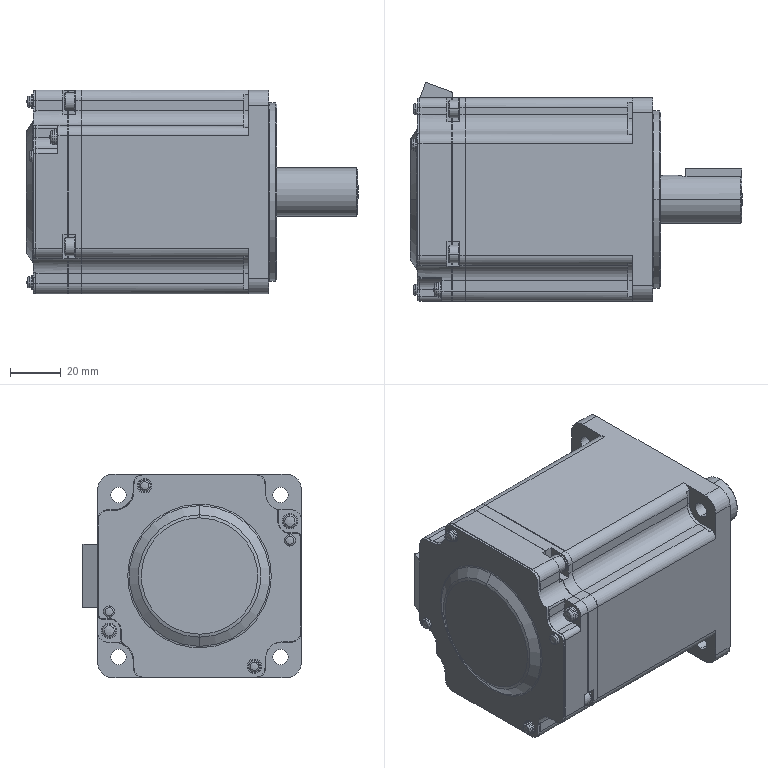Part | SolidWorks | features BaseBody 1 | 1 solid | 360 faces | box 130.4 x 85.907 x 80 mm | volume 551187 mm3 | plane 165 | cylinder 140 | cone 31 | spline 24 | commonest cylinder face diameters 8 x32 6 x13 7.84 x12 12 x10 7 x8 7.5 x6